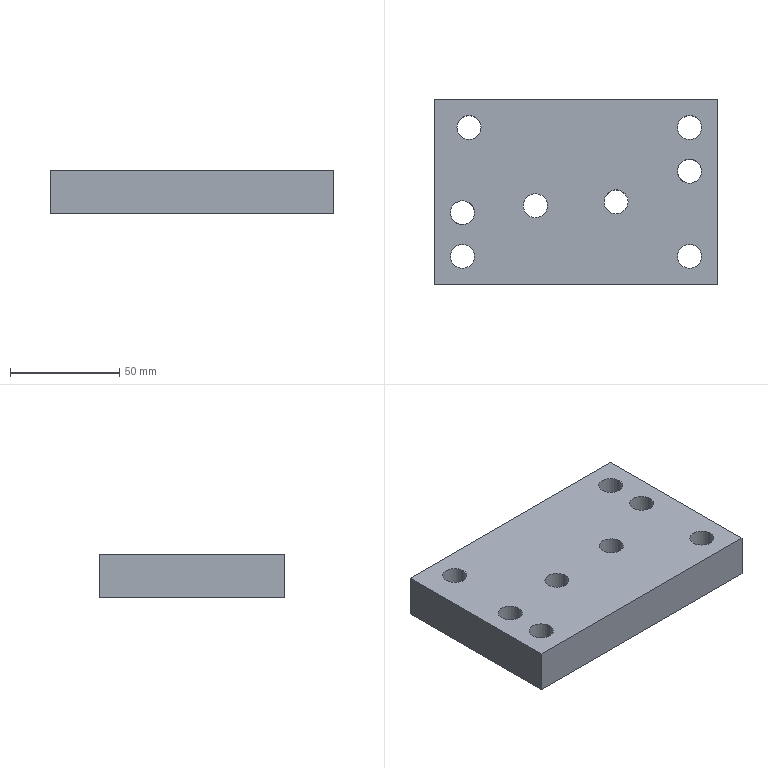Part | STEP file | 116_id2778_x_t | 1 solid | 14 faces | box 130 x 85 x 20 mm | volume 205795 mm3 | cylinder 8 | plane 6 | commonest cylinder face diameters 11 x8
STEP:
#1=CARTESIAN_POINT('',(0.,0.,0.));
#2=DIRECTION('',(0.,0.,1.));
#3=DIRECTION('',(1.,0.,0.));
#4=AXIS2_PLACEMENT_3D('',#1,#2,#3);
#5=CARTESIAN_POINT('',(1175.9,125.226,85.));
#6=VERTEX_POINT('',#5);
#7=CARTESIAN_POINT('',(1164.9,125.226,85.));
#8=VERTEX_POINT('',#7);
#9=CARTESIAN_POINT('',(1170.4,125.226,85.));
#10=DIRECTION('',(0.,0.,-1.));
#11=DIRECTION('',(-1.,0.,0.));
#12=AXIS2_PLACEMENT_3D('',#9,#10,#11);
#13=CIRCLE('',#12,5.5);
#14=CARTESIAN_POINT('',(1170.4,125.226,137.));
#15=DIRECTION('',(0.,0.,-1.));
#16=DIRECTION('',(1.,0.,0.));
#17=AXIS2_PLACEMENT_3D('',#14,#15,#16);
#18=CYLINDRICAL_SURFACE('',#17,5.5);
#19=CARTESIAN_POINT('',(-3.142,52.));
#20=DIRECTION('',(1.,0.));
#21=VECTOR('',#20,1.);
#22=LINE('',#19,#21);
#23=(GEOMETRIC_REPRESENTATION_CONTEXT(2)PARAMETRIC_REPRESENTATION_CONTEXT()REPRESENTATION_CONTEXT('',''));
#24=DEFINITIONAL_REPRESENTATION('',(#22),#23);
#25=PCURVE('',#18,#24);
#26=CARTESIAN_POINT('',(1128.,155.,85.));
#27=DIRECTION('',(0.,0.,-1.));
#28=DIRECTION('',(1.,0.,0.));
#29=AXIS2_PLACEMENT_3D('',#26,#27,#28);
#30=PLANE('',#29);
#31=CARTESIAN_POINT('',(42.4,29.774));
#32=DIRECTION('',(-1.,0.));
#33=AXIS2_PLACEMENT_2D('',#31,#32);
#34=CIRCLE('',#33,5.5);
#35=(GEOMETRIC_REPRESENTATION_CONTEXT(2)PARAMETRIC_REPRESENTATION_CONTEXT()REPRESENTATION_CONTEXT('',''));
#36=DEFINITIONAL_REPRESENTATION('',(#34),#35);
#37=PCURVE('',#30,#36);
#38=SURFACE_CURVE('',#13,(#25,#37),.PCURVE_S1.);
#39=EDGE_CURVE('',#6,#8,#38,.T.);
#40=ORIENTED_EDGE('',*,*,#39,.F.);
#41=CARTESIAN_POINT('',(1175.9,125.226,105.));
#42=VERTEX_POINT('',#41);
#43=CARTESIAN_POINT('',(1175.9,125.226,105.));
#44=CARTESIAN_POINT('',(1175.9,125.226,85.));
#45=B_SPLINE_CURVE_WITH_KNOTS('',1,(#43,#44),.UNSPECIFIED.,.F.,.F.,(2,2),(32.,52.),.PIECEWISE_BEZIER_KNOTS.);
#46=CARTESIAN_POINT('',(0.,0.));
#47=DIRECTION('',(0.,1.));
#48=VECTOR('',#47,1.);
#49=LINE('',#46,#48);
#50=(GEOMETRIC_REPRESENTATION_CONTEXT(2)PARAMETRIC_REPRESENTATION_CONTEXT()REPRESENTATION_CONTEXT('',''));
#51=DEFINITIONAL_REPRESENTATION('',(#49),#50);
#52=PCURVE('',#18,#51);
#53=CARTESIAN_POINT('',(6.283,0.));
#54=DIRECTION('',(0.,1.));
#55=VECTOR('',#54,1.);
#56=LINE('',#53,#55);
#57=(GEOMETRIC_REPRESENTATION_CONTEXT(2)PARAMETRIC_REPRESENTATION_CONTEXT()REPRESENTATION_CONTEXT('',''));
#58=DEFINITIONAL_REPRESENTATION('',(#56),#57);
#59=PCURVE('',#18,#58);
#60=SEAM_CURVE('',#45,(#52,#59),.PCURVE_S1.);
#61=EDGE_CURVE('',#42,#6,#60,.T.);
#62=ORIENTED_EDGE('',*,*,#61,.F.);
#63=CARTESIAN_POINT('',(1170.4,125.226,105.));
#64=DIRECTION('',(0.,0.,1.));
#65=DIRECTION('',(1.,0.,0.));
#66=AXIS2_PLACEMENT_3D('',#63,#64,#65);
#67=CIRCLE('',#66,5.5);
#68=CARTESIAN_POINT('',(6.283,32.));
#69=DIRECTION('',(-1.,0.));
#70=VECTOR('',#69,1.);
#71=LINE('',#68,#70);
#72=(GEOMETRIC_REPRESENTATION_CONTEXT(2)PARAMETRIC_REPRESENTATION_CONTEXT()REPRESENTATION_CONTEXT('',''));
#73=DEFINITIONAL_REPRESENTATION('',(#71),#72);
#74=PCURVE('',#18,#73);
#75=CARTESIAN_POINT('',(1128.,155.,105.));
#76=DIRECTION('',(0.,0.,1.));
#77=DIRECTION('',(-1.,0.,0.));
#78=AXIS2_PLACEMENT_3D('',#75,#76,#77);
#79=PLANE('',#78);
#80=CARTESIAN_POINT('',(-42.4,29.774));
#81=DIRECTION('',(-1.,0.));
#82=AXIS2_PLACEMENT_2D('',#80,#81);
#83=CIRCLE('',#82,5.5);
#84=(GEOMETRIC_REPRESENTATION_CONTEXT(2)PARAMETRIC_REPRESENTATION_CONTEXT()REPRESENTATION_CONTEXT('',''));
#85=DEFINITIONAL_REPRESENTATION('',(#83),#84);
#86=PCURVE('',#79,#85);
#87=SURFACE_CURVE('',#67,(#74,#86),.PCURVE_S1.);
#88=EDGE_CURVE('',#42,#42,#87,.T.);
#89=ORIENTED_EDGE('',*,*,#88,.F.);
#90=ORIENTED_EDGE('',*,*,#61,.T.);
#91=CARTESIAN_POINT('',(1170.4,125.226,85.));
#92=DIRECTION('',(0.,0.,-1.));
#93=DIRECTION('',(-1.,0.,0.));
#94=AXIS2_PLACEMENT_3D('',#91,#92,#93);
#95=CIRCLE('',#94,5.5);
#96=CARTESIAN_POINT('',(3.142,52.));
#97=DIRECTION('',(1.,0.));
#98=VECTOR('',#97,1.);
#99=LINE('',#96,#98);
#100=(GEOMETRIC_REPRESENTATION_CONTEXT(2)PARAMETRIC_REPRESENTATION_CONTEXT()REPRESENTATION_CONTEXT('',''));
#101=DEFINITIONAL_REPRESENTATION('',(#99),#100);
#102=PCURVE('',#18,#101);
#103=CARTESIAN_POINT('',(42.4,29.774));
#104=DIRECTION('',(-1.,0.));
#105=AXIS2_PLACEMENT_2D('',#103,#104);
#106=CIRCLE('',#105,5.5);
#107=(GEOMETRIC_REPRESENTATION_CONTEXT(2)PARAMETRIC_REPRESENTATION_CONTEXT()REPRESENTATION_CONTEXT('',''));
#108=DEFINITIONAL_REPRESENTATION('',(#106),#107);
#109=PCURVE('',#30,#108);
#110=SURFACE_CURVE('',#95,(#102,#109),.PCURVE_S1.);
#111=EDGE_CURVE('',#8,#6,#110,.T.);
#112=ORIENTED_EDGE('',*,*,#111,.F.);
#113=EDGE_LOOP('',(#40,#62,#89,#90,#112));
#114=FACE_BOUND('',#113,.F.);
#115=ADVANCED_FACE('',(#114),#18,.F.);
#116=CARTESIAN_POINT('',(1212.857,126.948,105.));
#117=VERTEX_POINT('',#116);
#118=CARTESIAN_POINT('',(1207.357,126.948,105.));
#119=DIRECTION('',(0.,0.,1.));
#120=DIRECTION('',(1.,0.,0.));
#121=AXIS2_PLACEMENT_3D('',#118,#119,#120);
#122=CIRCLE('',#121,5.5);
#123=CARTESIAN_POINT('',(1207.357,126.948,-13.));
#124=DIRECTION('',(0.,0.,1.));
#125=DIRECTION('',(0.9999,0.0167,0.));
#126=AXIS2_PLACEMENT_3D('',#123,#124,#125);
#127=CYLINDRICAL_SURFACE('',#126,5.5);
#128=CARTESIAN_POINT('',(6.266,118.));
#129=DIRECTION('',(1.,0.));
#130=VECTOR('',#129,1.);
#131=LINE('',#128,#130);
#132=(GEOMETRIC_REPRESENTATION_CONTEXT(2)PARAMETRIC_REPRESENTATION_CONTEXT()REPRESENTATION_CONTEXT('',''));
#133=DEFINITIONAL_REPRESENTATION('',(#131),#132);
#134=PCURVE('',#127,#133);
#135=CARTESIAN_POINT('',(-79.357,28.052));
#136=DIRECTION('',(-1.,0.));
#137=AXIS2_PLACEMENT_2D('',#135,#136);
#138=CIRCLE('',#137,5.5);
#139=(GEOMETRIC_REPRESENTATION_CONTEXT(2)PARAMETRIC_REPRESENTATION_CONTEXT()REPRESENTATION_CONTEXT('',''));
#140=DEFINITIONAL_REPRESENTATION('',(#138),#139);
#141=PCURVE('',#79,#140);
#142=SURFACE_CURVE('',#122,(#134,#141),.PCURVE_S1.);
#143=EDGE_CURVE('',#117,#117,#142,.T.);
#144=ORIENTED_EDGE('',*,*,#143,.F.);
#145=CARTESIAN_POINT('',(1212.857,126.948,85.));
#146=VERTEX_POINT('',#145);
#147=CARTESIAN_POINT('',(1212.857,126.948,85.));
#148=CARTESIAN_POINT('',(1212.857,126.948,105.));
#149=B_SPLINE_CURVE_WITH_KNOTS('',1,(#147,#148),.UNSPECIFIED.,.F.,.F.,(2,2),(98.,118.),.PIECEWISE_BEZIER_KNOTS.);
#150=CARTESIAN_POINT('',(6.266,0.));
#151=DIRECTION('',(0.,1.));
#152=VECTOR('',#151,1.);
#153=LINE('',#150,#152);
#154=(GEOMETRIC_REPRESENTATION_CONTEXT(2)PARAMETRIC_REPRESENTATION_CONTEXT()REPRESENTATION_CONTEXT('',''));
#155=DEFINITIONAL_REPRESENTATION('',(#153),#154);
#156=PCURVE('',#127,#155);
#157=CARTESIAN_POINT('',(12.55,0.));
#158=DIRECTION('',(0.,1.));
#159=VECTOR('',#158,1.);
#160=LINE('',#157,#159);
#161=(GEOMETRIC_REPRESENTATION_CONTEXT(2)PARAMETRIC_REPRESENTATION_CONTEXT()REPRESENTATION_CONTEXT('',''));
#162=DEFINITIONAL_REPRESENTATION('',(#160),#161);
#163=PCURVE('',#127,#162);
#164=SEAM_CURVE('',#149,(#156,#163),.PCURVE_S1.);
#165=EDGE_CURVE('',#146,#117,#164,.T.);
#166=ORIENTED_EDGE('',*,*,#165,.F.);
#167=CARTESIAN_POINT('',(1201.857,126.948,85.));
#168=VERTEX_POINT('',#167);
#169=CARTESIAN_POINT('',(1207.357,126.948,85.));
#170=DIRECTION('',(0.,0.,-1.));
#171=DIRECTION('',(-1.,0.,0.));
#172=AXIS2_PLACEMENT_3D('',#169,#170,#171);
#173=CIRCLE('',#172,5.5);
#174=CARTESIAN_POINT('',(9.408,98.));
#175=DIRECTION('',(-1.,0.));
#176=VECTOR('',#175,1.);
#177=LINE('',#174,#176);
#178=(GEOMETRIC_REPRESENTATION_CONTEXT(2)PARAMETRIC_REPRESENTATION_CONTEXT()REPRESENTATION_CONTEXT('',''));
#179=DEFINITIONAL_REPRESENTATION('',(#177),#178);
#180=PCURVE('',#127,#179);
#181=CARTESIAN_POINT('',(79.357,28.052));
#182=DIRECTION('',(-1.,0.));
#183=AXIS2_PLACEMENT_2D('',#181,#182);
#184=CIRCLE('',#183,5.5);
#185=(GEOMETRIC_REPRESENTATION_CONTEXT(2)PARAMETRIC_REPRESENTATION_CONTEXT()REPRESENTATION_CONTEXT('',''));
#186=DEFINITIONAL_REPRESENTATION('',(#184),#185);
#187=PCURVE('',#30,#186);
#188=SURFACE_CURVE('',#173,(#180,#187),.PCURVE_S1.);
#189=EDGE_CURVE('',#168,#146,#188,.T.);
#190=ORIENTED_EDGE('',*,*,#189,.F.);
#191=CARTESIAN_POINT('',(1207.357,126.948,85.));
#192=DIRECTION('',(0.,0.,-1.));
#193=DIRECTION('',(-1.,0.,0.));
#194=AXIS2_PLACEMENT_3D('',#191,#192,#193);
#195=CIRCLE('',#194,5.5);
#196=CARTESIAN_POINT('',(15.691,98.));
#197=DIRECTION('',(-1.,0.));
#198=VECTOR('',#197,1.);
#199=LINE('',#196,#198);
#200=(GEOMETRIC_REPRESENTATION_CONTEXT(2)PARAMETRIC_REPRESENTATION_CONTEXT()REPRESENTATION_CONTEXT('',''));
#201=DEFINITIONAL_REPRESENTATION('',(#199),#200);
#202=PCURVE('',#127,#201);
#203=CARTESIAN_POINT('',(79.357,28.052));
#204=DIRECTION('',(-1.,0.));
#205=AXIS2_PLACEMENT_2D('',#203,#204);
#206=CIRCLE('',#205,5.5);
#207=(GEOMETRIC_REPRESENTATION_CONTEXT(2)PARAMETRIC_REPRESENTATION_CONTEXT()REPRESENTATION_CONTEXT('',''));
#208=DEFINITIONAL_REPRESENTATION('',(#206),#207);
#209=PCURVE('',#30,#208);
#210=SURFACE_CURVE('',#195,(#202,#209),.PCURVE_S1.);
#211=EDGE_CURVE('',#146,#168,#210,.T.);
#212=ORIENTED_EDGE('',*,*,#211,.F.);
#213=ORIENTED_EDGE('',*,*,#165,.T.);
#214=EDGE_LOOP('',(#144,#166,#190,#212,#213));
#215=FACE_BOUND('',#214,.F.);
#216=ADVANCED_FACE('',(#215),#127,.F.);
#217=CARTESIAN_POINT('',(1124.,174.,105.));
#218=VERTEX_POINT('',#217);
#219=CARTESIAN_POINT('',(1254.,174.,105.));
#220=VERTEX_POINT('',#219);
#221=CARTESIAN_POINT('',(1128.,174.,105.));
#222=DIRECTION('',(1.,0.,0.));
#223=VECTOR('',#222,1.);
#224=LINE('',#221,#223);
#225=CARTESIAN_POINT('',(1128.,174.,90.));
#226=DIRECTION('',(0.,1.,0.));
#227=DIRECTION('',(0.,0.,-1.));
#228=AXIS2_PLACEMENT_3D('',#225,#226,#227);
#229=PLANE('',#228);
#230=CARTESIAN_POINT('',(-15.,0.));
#231=DIRECTION('',(0.,-1.));
#232=VECTOR('',#231,1.);
#233=LINE('',#230,#232);
#234=(GEOMETRIC_REPRESENTATION_CONTEXT(2)PARAMETRIC_REPRESENTATION_CONTEXT()REPRESENTATION_CONTEXT('',''));
#235=DEFINITIONAL_REPRESENTATION('',(#233),#234);
#236=PCURVE('',#229,#235);
#237=CARTESIAN_POINT('',(0.,-19.));
#238=DIRECTION('',(-1.,0.));
#239=VECTOR('',#238,1.);
#240=LINE('',#237,#239);
#241=(GEOMETRIC_REPRESENTATION_CONTEXT(2)PARAMETRIC_REPRESENTATION_CONTEXT()REPRESENTATION_CONTEXT('',''));
#242=DEFINITIONAL_REPRESENTATION('',(#240),#241);
#243=PCURVE('',#79,#242);
#244=SURFACE_CURVE('',#224,(#236,#243),.PCURVE_S1.);
#245=EDGE_CURVE('',#218,#220,#244,.T.);
#246=ORIENTED_EDGE('',*,*,#245,.T.);
#247=CARTESIAN_POINT('',(1254.,174.,85.));
#248=VERTEX_POINT('',#247);
#249=CARTESIAN_POINT('',(1254.,174.,90.));
#250=DIRECTION('',(0.,0.,1.));
#251=VECTOR('',#250,1.);
#252=LINE('',#249,#251);
#253=CARTESIAN_POINT('',(0.,-126.));
#254=DIRECTION('',(-1.,0.));
#255=VECTOR('',#254,1.);
#256=LINE('',#253,#255);
#257=(GEOMETRIC_REPRESENTATION_CONTEXT(2)PARAMETRIC_REPRESENTATION_CONTEXT()REPRESENTATION_CONTEXT('',''));
#258=DEFINITIONAL_REPRESENTATION('',(#256),#257);
#259=PCURVE('',#229,#258);
#260=CARTESIAN_POINT('',(1254.,155.,90.));
#261=DIRECTION('',(1.,0.,0.));
#262=DIRECTION('',(0.,0.,1.));
#263=AXIS2_PLACEMENT_3D('',#260,#261,#262);
#264=PLANE('',#263);
#265=CARTESIAN_POINT('',(0.,-19.));
#266=DIRECTION('',(1.,0.));
#267=VECTOR('',#266,1.);
#268=LINE('',#265,#267);
#269=(GEOMETRIC_REPRESENTATION_CONTEXT(2)PARAMETRIC_REPRESENTATION_CONTEXT()REPRESENTATION_CONTEXT('',''));
#270=DEFINITIONAL_REPRESENTATION('',(#268),#269);
#271=PCURVE('',#264,#270);
#272=SURFACE_CURVE('',#252,(#259,#271),.PCURVE_S1.);
#273=EDGE_CURVE('',#248,#220,#272,.T.);
#274=ORIENTED_EDGE('',*,*,#273,.F.);
#275=CARTESIAN_POINT('',(1124.,174.,85.));
#276=VERTEX_POINT('',#275);
#277=CARTESIAN_POINT('',(1128.,174.,85.));
#278=DIRECTION('',(-1.,0.,0.));
#279=VECTOR('',#278,1.);
#280=LINE('',#277,#279);
#281=CARTESIAN_POINT('',(5.,0.));
#282=DIRECTION('',(0.,1.));
#283=VECTOR('',#282,1.);
#284=LINE('',#281,#283);
#285=(GEOMETRIC_REPRESENTATION_CONTEXT(2)PARAMETRIC_REPRESENTATION_CONTEXT()REPRESENTATION_CONTEXT('',''));
#286=DEFINITIONAL_REPRESENTATION('',(#284),#285);
#287=PCURVE('',#229,#286);
#288=CARTESIAN_POINT('',(0.,-19.));
#289=DIRECTION('',(-1.,0.));
#290=VECTOR('',#289,1.);
#291=LINE('',#288,#290);
#292=(GEOMETRIC_REPRESENTATION_CONTEXT(2)PARAMETRIC_REPRESENTATION_CONTEXT()REPRESENTATION_CONTEXT('',''));
#293=DEFINITIONAL_REPRESENTATION('',(#291),#292);
#294=PCURVE('',#30,#293);
#295=SURFACE_CURVE('',#280,(#287,#294),.PCURVE_S1.);
#296=EDGE_CURVE('',#248,#276,#295,.T.);
#297=ORIENTED_EDGE('',*,*,#296,.T.);
#298=CARTESIAN_POINT('',(1124.,174.,90.));
#299=DIRECTION('',(0.,0.,-1.));
#300=VECTOR('',#299,1.);
#301=LINE('',#298,#300);
#302=CARTESIAN_POINT('',(0.,4.));
#303=DIRECTION('',(1.,0.));
#304=VECTOR('',#303,1.);
#305=LINE('',#302,#304);
#306=(GEOMETRIC_REPRESENTATION_CONTEXT(2)PARAMETRIC_REPRESENTATION_CONTEXT()REPRESENTATION_CONTEXT('',''));
#307=DEFINITIONAL_REPRESENTATION('',(#305),#306);
#308=PCURVE('',#229,#307);
#309=CARTESIAN_POINT('',(1124.,108.,90.));
#310=DIRECTION('',(-1.,0.,0.));
#311=DIRECTION('',(0.,0.,1.));
#312=AXIS2_PLACEMENT_3D('',#309,#310,#311);
#313=PLANE('',#312);
#314=CARTESIAN_POINT('',(0.,66.));
#315=DIRECTION('',(-1.,0.));
#316=VECTOR('',#315,1.);
#317=LINE('',#314,#316);
#318=(GEOMETRIC_REPRESENTATION_CONTEXT(2)PARAMETRIC_REPRESENTATION_CONTEXT()REPRESENTATION_CONTEXT('',''));
#319=DEFINITIONAL_REPRESENTATION('',(#317),#318);
#320=PCURVE('',#313,#319);
#321=SURFACE_CURVE('',#301,(#308,#320),.PCURVE_S1.);
#322=EDGE_CURVE('',#218,#276,#321,.T.);
#323=ORIENTED_EDGE('',*,*,#322,.F.);
#324=EDGE_LOOP('',(#246,#274,#297,#323));
#325=FACE_BOUND('',#324,.T.);
#326=ADVANCED_FACE('',(#325),#229,.T.);
#327=CARTESIAN_POINT('',(1124.,89.,85.));
#328=VERTEX_POINT('',#327);
#329=CARTESIAN_POINT('',(1254.,89.,85.));
#330=VERTEX_POINT('',#329);
#331=CARTESIAN_POINT('',(1128.,89.,85.));
#332=DIRECTION('',(1.,0.,0.));
#333=VECTOR('',#332,1.);
#334=LINE('',#331,#333);
#335=CARTESIAN_POINT('',(1128.,89.,90.));
#336=DIRECTION('',(0.,-1.,0.));
#337=DIRECTION('',(0.,0.,1.));
#338=AXIS2_PLACEMENT_3D('',#335,#336,#337);
#339=PLANE('',#338);
#340=CARTESIAN_POINT('',(-5.,0.));
#341=DIRECTION('',(0.,-1.));
#342=VECTOR('',#341,1.);
#343=LINE('',#340,#342);
#344=(GEOMETRIC_REPRESENTATION_CONTEXT(2)PARAMETRIC_REPRESENTATION_CONTEXT()REPRESENTATION_CONTEXT('',''));
#345=DEFINITIONAL_REPRESENTATION('',(#343),#344);
#346=PCURVE('',#339,#345);
#347=CARTESIAN_POINT('',(0.,66.));
#348=DIRECTION('',(1.,0.));
#349=VECTOR('',#348,1.);
#350=LINE('',#347,#349);
#351=(GEOMETRIC_REPRESENTATION_CONTEXT(2)PARAMETRIC_REPRESENTATION_CONTEXT()REPRESENTATION_CONTEXT('',''));
#352=DEFINITIONAL_REPRESENTATION('',(#350),#351);
#353=PCURVE('',#30,#352);
#354=SURFACE_CURVE('',#334,(#346,#353),.PCURVE_S1.);
#355=EDGE_CURVE('',#328,#330,#354,.T.);
#356=ORIENTED_EDGE('',*,*,#355,.T.);
#357=CARTESIAN_POINT('',(1254.,89.,105.));
#358=VERTEX_POINT('',#357);
#359=CARTESIAN_POINT('',(1254.,89.,90.));
#360=DIRECTION('',(0.,0.,1.));
#361=VECTOR('',#360,1.);
#362=LINE('',#359,#361);
#363=CARTESIAN_POINT('',(0.,-126.));
#364=DIRECTION('',(1.,0.));
#365=VECTOR('',#364,1.);
#366=LINE('',#363,#365);
#367=(GEOMETRIC_REPRESENTATION_CONTEXT(2)PARAMETRIC_REPRESENTATION_CONTEXT()REPRESENTATION_CONTEXT('',''));
#368=DEFINITIONAL_REPRESENTATION('',(#366),#367);
#369=PCURVE('',#339,#368);
#370=CARTESIAN_POINT('',(0.,66.));
#371=DIRECTION('',(1.,0.));
#372=VECTOR('',#371,1.);
#373=LINE('',#370,#372);
#374=(GEOMETRIC_REPRESENTATION_CONTEXT(2)PARAMETRIC_REPRESENTATION_CONTEXT()REPRESENTATION_CONTEXT('',''));
#375=DEFINITIONAL_REPRESENTATION('',(#373),#374);
#376=PCURVE('',#264,#375);
#377=SURFACE_CURVE('',#362,(#369,#376),.PCURVE_S1.);
#378=EDGE_CURVE('',#330,#358,#377,.T.);
#379=ORIENTED_EDGE('',*,*,#378,.T.);
#380=CARTESIAN_POINT('',(1124.,89.,105.));
#381=VERTEX_POINT('',#380);
#382=CARTESIAN_POINT('',(1128.,89.,105.));
#383=DIRECTION('',(-1.,0.,0.));
#384=VECTOR('',#383,1.);
#385=LINE('',#382,#384);
#386=CARTESIAN_POINT('',(15.,0.));
#387=DIRECTION('',(0.,1.));
#388=VECTOR('',#387,1.);
#389=LINE('',#386,#388);
#390=(GEOMETRIC_REPRESENTATION_CONTEXT(2)PARAMETRIC_REPRESENTATION_CONTEXT()REPRESENTATION_CONTEXT('',''));
#391=DEFINITIONAL_REPRESENTATION('',(#389),#390);
#392=PCURVE('',#339,#391);
#393=CARTESIAN_POINT('',(0.,66.));
#394=DIRECTION('',(1.,0.));
#395=VECTOR('',#394,1.);
#396=LINE('',#393,#395);
#397=(GEOMETRIC_REPRESENTATION_CONTEXT(2)PARAMETRIC_REPRESENTATION_CONTEXT()REPRESENTATION_CONTEXT('',''));
#398=DEFINITIONAL_REPRESENTATION('',(#396),#397);
#399=PCURVE('',#79,#398);
#400=SURFACE_CURVE('',#385,(#392,#399),.PCURVE_S1.);
#401=EDGE_CURVE('',#358,#381,#400,.T.);
#402=ORIENTED_EDGE('',*,*,#401,.T.);
#403=CARTESIAN_POINT('',(1124.,89.,90.));
#404=DIRECTION('',(0.,0.,-1.));
#405=VECTOR('',#404,1.);
#406=LINE('',#403,#405);
#407=CARTESIAN_POINT('',(0.,4.));
#408=DIRECTION('',(-1.,0.));
#409=VECTOR('',#408,1.);
#410=LINE('',#407,#409);
#411=(GEOMETRIC_REPRESENTATION_CONTEXT(2)PARAMETRIC_REPRESENTATION_CONTEXT()REPRESENTATION_CONTEXT('',''));
#412=DEFINITIONAL_REPRESENTATION('',(#410),#411);
#413=PCURVE('',#339,#412);
#414=CARTESIAN_POINT('',(0.,-19.));
#415=DIRECTION('',(-1.,0.));
#416=VECTOR('',#415,1.);
#417=LINE('',#414,#416);
#418=(GEOMETRIC_REPRESENTATION_CONTEXT(2)PARAMETRIC_REPRESENTATION_CONTEXT()REPRESENTATION_CONTEXT('',''));
#419=DEFINITIONAL_REPRESENTATION('',(#417),#418);
#420=PCURVE('',#313,#419);
#421=SURFACE_CURVE('',#406,(#413,#420),.PCURVE_S1.);
#422=EDGE_CURVE('',#381,#328,#421,.T.);
#423=ORIENTED_EDGE('',*,*,#422,.T.);
#424=EDGE_LOOP('',(#356,#379,#402,#423));
#425=FACE_BOUND('',#424,.T.);
#426=ADVANCED_FACE('',(#425),#339,.T.);
#427=ORIENTED_EDGE('',*,*,#143,.F.);
#428=EDGE_LOOP('',(#427));
#429=FACE_BOUND('',#428,.T.);
#430=ORIENTED_EDGE('',*,*,#88,.F.);
#431=EDGE_LOOP('',(#430));
#432=FACE_BOUND('',#431,.T.);
#433=ORIENTED_EDGE('',*,*,#401,.F.);
#434=CARTESIAN_POINT('',(1254.,155.,105.));
#435=DIRECTION('',(0.,-1.,0.));
#436=VECTOR('',#435,1.);
#437=LINE('',#434,#436);
#438=CARTESIAN_POINT('',(-126.,0.));
#439=DIRECTION('',(0.,1.));
#440=VECTOR('',#439,1.);
#441=LINE('',#438,#440);
#442=(GEOMETRIC_REPRESENTATION_CONTEXT(2)PARAMETRIC_REPRESENTATION_CONTEXT()REPRESENTATION_CONTEXT('',''));
#443=DEFINITIONAL_REPRESENTATION('',(#441),#442);
#444=PCURVE('',#79,#443);
#445=CARTESIAN_POINT('',(15.,0.));
#446=DIRECTION('',(0.,1.));
#447=VECTOR('',#446,1.);
#448=LINE('',#445,#447);
#449=(GEOMETRIC_REPRESENTATION_CONTEXT(2)PARAMETRIC_REPRESENTATION_CONTEXT()REPRESENTATION_CONTEXT('',''));
#450=DEFINITIONAL_REPRESENTATION('',(#448),#449);
#451=PCURVE('',#264,#450);
#452=SURFACE_CURVE('',#437,(#444,#451),.PCURVE_S1.);
#453=EDGE_CURVE('',#220,#358,#452,.T.);
#454=ORIENTED_EDGE('',*,*,#453,.F.);
#455=ORIENTED_EDGE('',*,*,#245,.F.);
#456=CARTESIAN_POINT('',(1124.,155.,105.));
#457=DIRECTION('',(0.,-1.,0.));
#458=VECTOR('',#457,1.);
#459=LINE('',#456,#458);
#460=CARTESIAN_POINT('',(4.,0.));
#461=DIRECTION('',(0.,1.));
#462=VECTOR('',#461,1.);
#463=LINE('',#460,#462);
#464=(GEOMETRIC_REPRESENTATION_CONTEXT(2)PARAMETRIC_REPRESENTATION_CONTEXT()REPRESENTATION_CONTEXT('',''));
#465=DEFINITIONAL_REPRESENTATION('',(#463),#464);
#466=PCURVE('',#79,#465);
#467=CARTESIAN_POINT('',(15.,47.));
#468=DIRECTION('',(0.,-1.));
#469=VECTOR('',#468,1.);
#470=LINE('',#467,#469);
#471=(GEOMETRIC_REPRESENTATION_CONTEXT(2)PARAMETRIC_REPRESENTATION_CONTEXT()REPRESENTATION_CONTEXT('',''));
#472=DEFINITIONAL_REPRESENTATION('',(#470),#471);
#473=PCURVE('',#313,#472);
#474=SURFACE_CURVE('',#459,(#466,#473),.PCURVE_S1.);
#475=EDGE_CURVE('',#218,#381,#474,.T.);
#476=ORIENTED_EDGE('',*,*,#475,.T.);
#477=EDGE_LOOP('',(#433,#454,#455,#476));
#478=FACE_BOUND('',#477,.T.);
#479=CARTESIAN_POINT('',(1134.5,161.,105.));
#480=VERTEX_POINT('',#479);
#481=CARTESIAN_POINT('',(1140.,161.,105.));
#482=DIRECTION('',(0.,0.,1.));
#483=DIRECTION('',(1.,0.,0.));
#484=AXIS2_PLACEMENT_3D('',#481,#482,#483);
#485=CIRCLE('',#484,5.5);
#486=CARTESIAN_POINT('',(-12.,-6.));
#487=DIRECTION('',(-1.,0.));
#488=AXIS2_PLACEMENT_2D('',#486,#487);
#489=CIRCLE('',#488,5.5);
#490=(GEOMETRIC_REPRESENTATION_CONTEXT(2)PARAMETRIC_REPRESENTATION_CONTEXT()REPRESENTATION_CONTEXT('',''));
#491=DEFINITIONAL_REPRESENTATION('',(#489),#490);
#492=PCURVE('',#79,#491);
#493=CARTESIAN_POINT('',(1140.,161.,90.));
#494=DIRECTION('',(0.,0.,1.));
#495=DIRECTION('',(1.,0.,0.));
#496=AXIS2_PLACEMENT_3D('',#493,#494,#495);
#497=CYLINDRICAL_SURFACE('',#496,5.5);
#498=CARTESIAN_POINT('',(0.,15.));
#499=DIRECTION('',(1.,0.));
#500=VECTOR('',#499,1.);
#501=LINE('',#498,#500);
#502=(GEOMETRIC_REPRESENTATION_CONTEXT(2)PARAMETRIC_REPRESENTATION_CONTEXT()REPRESENTATION_CONTEXT('',''));
#503=DEFINITIONAL_REPRESENTATION('',(#501),#502);
#504=PCURVE('',#497,#503);
#505=SURFACE_CURVE('',#485,(#492,#504),.PCURVE_S1.);
#506=EDGE_CURVE('',#480,#480,#505,.T.);
#507=ORIENTED_EDGE('',*,*,#506,.F.);
#508=EDGE_LOOP('',(#507));
#509=FACE_BOUND('',#508,.T.);
#510=CARTESIAN_POINT('',(1131.5,102.,105.));
#511=VERTEX_POINT('',#510);
#512=CARTESIAN_POINT('',(1137.,102.,105.));
#513=DIRECTION('',(0.,0.,1.));
#514=DIRECTION('',(1.,0.,0.));
#515=AXIS2_PLACEMENT_3D('',#512,#513,#514);
#516=CIRCLE('',#515,5.5);
#517=CARTESIAN_POINT('',(-9.,53.));
#518=DIRECTION('',(-1.,0.));
#519=AXIS2_PLACEMENT_2D('',#517,#518);
#520=CIRCLE('',#519,5.5);
#521=(GEOMETRIC_REPRESENTATION_CONTEXT(2)PARAMETRIC_REPRESENTATION_CONTEXT()REPRESENTATION_CONTEXT('',''));
#522=DEFINITIONAL_REPRESENTATION('',(#520),#521);
#523=PCURVE('',#79,#522);
#524=CARTESIAN_POINT('',(1137.,102.,90.));
#525=DIRECTION('',(0.,0.,1.));
#526=DIRECTION('',(1.,0.,0.));
#527=AXIS2_PLACEMENT_3D('',#524,#525,#526);
#528=CYLINDRICAL_SURFACE('',#527,5.5);
#529=CARTESIAN_POINT('',(0.,15.));
#530=DIRECTION('',(1.,0.));
#531=VECTOR('',#530,1.);
#532=LINE('',#529,#531);
#533=(GEOMETRIC_REPRESENTATION_CONTEXT(2)PARAMETRIC_REPRESENTATION_CONTEXT()REPRESENTATION_CONTEXT('',''));
#534=DEFINITIONAL_REPRESENTATION('',(#532),#533);
#535=PCURVE('',#528,#534);
#536=SURFACE_CURVE('',#516,(#523,#535),.PCURVE_S1.);
#537=EDGE_CURVE('',#511,#511,#536,.T.);
#538=ORIENTED_EDGE('',*,*,#537,.F.);
#539=EDGE_LOOP('',(#538));
#540=FACE_BOUND('',#539,.T.);
#541=CARTESIAN_POINT('',(1131.5,122.,105.));
#542=VERTEX_POINT('',#541);
#543=CARTESIAN_POINT('',(1137.,122.,105.));
#544=DIRECTION('',(0.,0.,1.));
#545=DIRECTION('',(1.,0.,0.));
#546=AXIS2_PLACEMENT_3D('',#543,#544,#545);
#547=CIRCLE('',#546,5.5);
#548=CARTESIAN_POINT('',(-9.,33.));
#549=DIRECTION('',(-1.,0.));
#550=AXIS2_PLACEMENT_2D('',#548,#549);
#551=CIRCLE('',#550,5.5);
#552=(GEOMETRIC_REPRESENTATION_CONTEXT(2)PARAMETRIC_REPRESENTATION_CONTEXT()REPRESENTATION_CONTEXT('',''));
#553=DEFINITIONAL_REPRESENTATION('',(#551),#552);
#554=PCURVE('',#79,#553);
#555=CARTESIAN_POINT('',(1137.,122.,90.));
#556=DIRECTION('',(0.,0.,1.));
#557=DIRECTION('',(0.,1.,0.));
#558=AXIS2_PLACEMENT_3D('',#555,#556,#557);
#559=CYLINDRICAL_SURFACE('',#558,5.5);
#560=CARTESIAN_POINT('',(-1.571,15.));
#561=DIRECTION('',(1.,0.));
#562=VECTOR('',#561,1.);
#563=LINE('',#560,#562);
#564=(GEOMETRIC_REPRESENTATION_CONTEXT(2)PARAMETRIC_REPRESENTATION_CONTEXT()REPRESENTATION_CONTEXT('',''));
#565=DEFINITIONAL_REPRESENTATION('',(#563),#564);
#566=PCURVE('',#559,#565);
#567=SURFACE_CURVE('',#547,(#554,#566),.PCURVE_S1.);
#568=EDGE_CURVE('',#542,#542,#567,.T.);
#569=ORIENTED_EDGE('',*,*,#568,.F.);
#570=EDGE_LOOP('',(#569));
#571=FACE_BOUND('',#570,.T.);
#572=CARTESIAN_POINT('',(1246.5,102.,105.));
#573=VERTEX_POINT('',#572);
#574=CARTESIAN_POINT('',(1241.,102.,105.));
#575=DIRECTION('',(0.,0.,-1.));
#576=DIRECTION('',(1.,0.,0.));
#577=AXIS2_PLACEMENT_3D('',#574,#575,#576);
#578=CIRCLE('',#577,5.5);
#579=CARTESIAN_POINT('',(-118.5,53.));
#580=CARTESIAN_POINT('',(-118.5,62.526));
#581=CARTESIAN_POINT('',(-110.25,57.763));
#582=CARTESIAN_POINT('',(-102.,53.));
#583=CARTESIAN_POINT('',(-110.25,48.237));
#584=CARTESIAN_POINT('',(-118.5,43.474));
#585=CARTESIAN_POINT('',(-118.5,53.));
#586=(BOUNDED_CURVE()B_SPLINE_CURVE(2,(#579,#580,#581,#582,#583,#584,#585),.UNSPECIFIED.,.T.,.F.)B_SPLINE_CURVE_WITH_KNOTS((1,2,2,2,2,1),(-2.094,0.,2.094,4.189,6.283,8.378),.UNSPECIFIED.)CURVE()GEOMETRIC_REPRESENTATION_ITEM()RATIONAL_B_SPLINE_CURVE((1.,0.5,1.,0.5,1.,0.5,1.))REPRESENTATION_ITEM(''));
#587=(GEOMETRIC_REPRESENTATION_CONTEXT(2)PARAMETRIC_REPRESENTATION_CONTEXT()REPRESENTATION_CONTEXT('',''));
#588=DEFINITIONAL_REPRESENTATION('',(#586),#587);
#589=PCURVE('',#79,#588);
#590=CARTESIAN_POINT('',(1241.,102.,90.));
#591=DIRECTION('',(0.,0.,1.));
#592=DIRECTION('',(-1.,0.,0.));
#593=AXIS2_PLACEMENT_3D('',#590,#591,#592);
#594=CYLINDRICAL_SURFACE('',#593,5.5);
#595=CARTESIAN_POINT('',(9.425,15.));
#596=DIRECTION('',(-1.,0.));
#597=VECTOR('',#596,1.);
#598=LINE('',#595,#597);
#599=(GEOMETRIC_REPRESENTATION_CONTEXT(2)PARAMETRIC_REPRESENTATION_CONTEXT()REPRESENTATION_CONTEXT('',''));
#600=DEFINITIONAL_REPRESENTATION('',(#598),#599);
#601=PCURVE('',#594,#600);
#602=SURFACE_CURVE('',#578,(#589,#601),.PCURVE_S1.);
#603=EDGE_CURVE('',#573,#573,#602,.T.);
#604=ORIENTED_EDGE('',*,*,#603,.T.);
#605=EDGE_LOOP('',(#604));
#606=FACE_BOUND('',#605,.T.);
#607=CARTESIAN_POINT('',(1246.5,161.,105.));
#608=VERTEX_POINT('',#607);
#609=CARTESIAN_POINT('',(1241.,161.,105.));
#610=DIRECTION('',(0.,0.,-1.));
#611=DIRECTION('',(1.,0.,0.));
#612=AXIS2_PLACEMENT_3D('',#609,#610,#611);
#613=CIRCLE('',#612,5.5);
#614=CARTESIAN_POINT('',(-118.5,-6.));
#615=CARTESIAN_POINT('',(-118.5,3.526));
#616=CARTESIAN_POINT('',(-110.25,-1.237));
#617=CARTESIAN_POINT('',(-102.,-6.));
#618=CARTESIAN_POINT('',(-110.25,-10.763));
#619=CARTESIAN_POINT('',(-118.5,-15.526));
#620=CARTESIAN_POINT('',(-118.5,-6.));
#621=(BOUNDED_CURVE()B_SPLINE_CURVE(2,(#614,#615,#616,#617,#618,#619,#620),.UNSPECIFIED.,.T.,.F.)B_SPLINE_CURVE_WITH_KNOTS((1,2,2,2,2,1),(-2.094,0.,2.094,4.189,6.283,8.378),.UNSPECIFIED.)CURVE()GEOMETRIC_REPRESENTATION_ITEM()RATIONAL_B_SPLINE_CURVE((1.,0.5,1.,0.5,1.,0.5,1.))REPRESENTATION_ITEM(''));
#622=(GEOMETRIC_REPRESENTATION_CONTEXT(2)PARAMETRIC_REPRESENTATION_CONTEXT()REPRESENTATION_CONTEXT('',''));
#623=DEFINITIONAL_REPRESENTATION('',(#621),#622);
#624=PCURVE('',#79,#623);
#625=CARTESIAN_POINT('',(1241.,161.,90.));
#626=DIRECTION('',(0.,0.,1.));
#627=DIRECTION('',(-1.,0.,0.));
#628=AXIS2_PLACEMENT_3D('',#625,#626,#627);
#629=CYLINDRICAL_SURFACE('',#628,5.5);
#630=CARTESIAN_POINT('',(9.425,15.));
#631=DIRECTION('',(-1.,0.));
#632=VECTOR('',#631,1.);
#633=LINE('',#630,#632);
#634=(GEOMETRIC_REPRESENTATION_CONTEXT(2)PARAMETRIC_REPRESENTATION_CONTEXT()REPRESENTATION_CONTEXT('',''));
#635=DEFINITIONAL_REPRESENTATION('',(#633),#634);
#636=PCURVE('',#629,#635);
#637=SURFACE_CURVE('',#613,(#624,#636),.PCURVE_S1.);
#638=EDGE_CURVE('',#608,#608,#637,.T.);
#639=ORIENTED_EDGE('',*,*,#638,.T.);
#640=EDGE_LOOP('',(#639));
#641=FACE_BOUND('',#640,.T.);
#642=CARTESIAN_POINT('',(1246.5,141.,105.));
#643=VERTEX_POINT('',#642);
#644=CARTESIAN_POINT('',(1241.,141.,105.));
#645=DIRECTION('',(0.,0.,-1.));
#646=DIRECTION('',(1.,0.,0.));
#647=AXIS2_PLACEMENT_3D('',#644,#645,#646);
#648=CIRCLE('',#647,5.5);
#649=CARTESIAN_POINT('',(-118.5,14.));
#650=CARTESIAN_POINT('',(-118.5,23.526));
#651=CARTESIAN_POINT('',(-110.25,18.763));
#652=CARTESIAN_POINT('',(-102.,14.));
#653=CARTESIAN_POINT('',(-110.25,9.237));
#654=CARTESIAN_POINT('',(-118.5,4.474));
#655=CARTESIAN_POINT('',(-118.5,14.));
#656=(BOUNDED_CURVE()B_SPLINE_CURVE(2,(#649,#650,#651,#652,#653,#654,#655),.UNSPECIFIED.,.T.,.F.)B_SPLINE_CURVE_WITH_KNOTS((1,2,2,2,2,1),(-2.094,0.,2.094,4.189,6.283,8.378),.UNSPECIFIED.)CURVE()GEOMETRIC_REPRESENTATION_ITEM()RATIONAL_B_SPLINE_CURVE((1.,0.5,1.,0.5,1.,0.5,1.))REPRESENTATION_ITEM(''));
#657=(GEOMETRIC_REPRESENTATION_CONTEXT(2)PARAMETRIC_REPRESENTATION_CONTEXT()REPRESENTATION_CONTEXT('',''));
#658=DEFINITIONAL_REPRESENTATION('',(#656),#657);
#659=PCURVE('',#79,#658);
#660=CARTESIAN_POINT('',(1241.,141.,90.));
#661=DIRECTION('',(0.,0.,1.));
#662=DIRECTION('',(0.,-1.,0.));
#663=AXIS2_PLACEMENT_3D('',#660,#661,#662);
#664=CYLINDRICAL_SURFACE('',#663,5.5);
#665=CARTESIAN_POINT('',(7.854,15.));
#666=DIRECTION('',(-1.,0.));
#667=VECTOR('',#666,1.);
#668=LINE('',#665,#667);
#669=(GEOMETRIC_REPRESENTATION_CONTEXT(2)PARAMETRIC_REPRESENTATION_CONTEXT()REPRESENTATION_CONTEXT('',''));
#670=DEFINITIONAL_REPRESENTATION('',(#668),#669);
#671=PCURVE('',#664,#670);
#672=SURFACE_CURVE('',#648,(#659,#671),.PCURVE_S1.);
#673=EDGE_CURVE('',#643,#643,#672,.T.);
#674=ORIENTED_EDGE('',*,*,#673,.T.);
#675=EDGE_LOOP('',(#674));
#676=FACE_BOUND('',#675,.T.);
#677=ADVANCED_FACE('',(#429,#432,#478,#509,#540,#571,#606,#641,#676),#79,.T.);
#678=ORIENTED_EDGE('',*,*,#189,.F.);
#679=ORIENTED_EDGE('',*,*,#211,.F.);
#680=EDGE_LOOP('',(#678,#679));
#681=FACE_BOUND('',#680,.T.);
#682=ORIENTED_EDGE('',*,*,#111,.F.);
#683=ORIENTED_EDGE('',*,*,#39,.F.);
#684=EDGE_LOOP('',(#682,#683));
#685=FACE_BOUND('',#684,.T.);
#686=ORIENTED_EDGE('',*,*,#296,.F.);
#687=CARTESIAN_POINT('',(1254.,155.,85.));
#688=DIRECTION('',(0.,1.,0.));
#689=VECTOR('',#688,1.);
#690=LINE('',#687,#689);
#691=CARTESIAN_POINT('',(126.,0.));
#692=DIRECTION('',(0.,-1.));
#693=VECTOR('',#692,1.);
#694=LINE('',#691,#693);
#695=(GEOMETRIC_REPRESENTATION_CONTEXT(2)PARAMETRIC_REPRESENTATION_CONTEXT()REPRESENTATION_CONTEXT('',''));
#696=DEFINITIONAL_REPRESENTATION('',(#694),#695);
#697=PCURVE('',#30,#696);
#698=CARTESIAN_POINT('',(-5.,0.));
#699=DIRECTION('',(0.,-1.));
#700=VECTOR('',#699,1.);
#701=LINE('',#698,#700);
#702=(GEOMETRIC_REPRESENTATION_CONTEXT(2)PARAMETRIC_REPRESENTATION_CONTEXT()REPRESENTATION_CONTEXT('',''));
#703=DEFINITIONAL_REPRESENTATION('',(#701),#702);
#704=PCURVE('',#264,#703);
#705=SURFACE_CURVE('',#690,(#697,#704),.PCURVE_S1.);
#706=EDGE_CURVE('',#330,#248,#705,.T.);
#707=ORIENTED_EDGE('',*,*,#706,.F.);
#708=ORIENTED_EDGE('',*,*,#355,.F.);
#709=CARTESIAN_POINT('',(1124.,155.,85.));
#710=DIRECTION('',(0.,1.,0.));
#711=VECTOR('',#710,1.);
#712=LINE('',#709,#711);
#713=CARTESIAN_POINT('',(-4.,0.));
#714=DIRECTION('',(0.,-1.));
#715=VECTOR('',#714,1.);
#716=LINE('',#713,#715);
#717=(GEOMETRIC_REPRESENTATION_CONTEXT(2)PARAMETRIC_REPRESENTATION_CONTEXT()REPRESENTATION_CONTEXT('',''));
#718=DEFINITIONAL_REPRESENTATION('',(#716),#717);
#719=PCURVE('',#30,#718);
#720=CARTESIAN_POINT('',(-5.,47.));
#721=DIRECTION('',(0.,1.));
#722=VECTOR('',#721,1.);
#723=LINE('',#720,#722);
#724=(GEOMETRIC_REPRESENTATION_CONTEXT(2)PARAMETRIC_REPRESENTATION_CONTEXT()REPRESENTATION_CONTEXT('',''));
#725=DEFINITIONAL_REPRESENTATION('',(#723),#724);
#726=PCURVE('',#313,#725);
#727=SURFACE_CURVE('',#712,(#719,#726),.PCURVE_S1.);
#728=EDGE_CURVE('',#328,#276,#727,.T.);
#729=ORIENTED_EDGE('',*,*,#728,.T.);
#730=EDGE_LOOP('',(#686,#707,#708,#729));
#731=FACE_BOUND('',#730,.T.);
#732=CARTESIAN_POINT('',(1131.5,102.,85.));
#733=VERTEX_POINT('',#732);
#734=CARTESIAN_POINT('',(1137.,102.,85.));
#735=DIRECTION('',(0.,0.,-1.));
#736=DIRECTION('',(-1.,0.,0.));
#737=AXIS2_PLACEMENT_3D('',#734,#735,#736);
#738=CIRCLE('',#737,5.5);
#739=CARTESIAN_POINT('',(9.,53.));
#740=DIRECTION('',(-1.,0.));
#741=AXIS2_PLACEMENT_2D('',#739,#740);
#742=CIRCLE('',#741,5.5);
#743=(GEOMETRIC_REPRESENTATION_CONTEXT(2)PARAMETRIC_REPRESENTATION_CONTEXT()REPRESENTATION_CONTEXT('',''));
#744=DEFINITIONAL_REPRESENTATION('',(#742),#743);
#745=PCURVE('',#30,#744);
#746=CARTESIAN_POINT('',(9.425,-5.));
#747=DIRECTION('',(-1.,0.));
#748=VECTOR('',#747,1.);
#749=LINE('',#746,#748);
#750=(GEOMETRIC_REPRESENTATION_CONTEXT(2)PARAMETRIC_REPRESENTATION_CONTEXT()REPRESENTATION_CONTEXT('',''));
#751=DEFINITIONAL_REPRESENTATION('',(#749),#750);
#752=PCURVE('',#528,#751);
#753=SURFACE_CURVE('',#738,(#745,#752),.PCURVE_S1.);
#754=EDGE_CURVE('',#733,#733,#753,.T.);
#755=ORIENTED_EDGE('',*,*,#754,.F.);
#756=EDGE_LOOP('',(#755));
#757=FACE_BOUND('',#756,.T.);
#758=CARTESIAN_POINT('',(1137.,116.5,85.));
#759=VERTEX_POINT('',#758);
#760=CARTESIAN_POINT('',(1131.5,122.,85.));
#761=VERTEX_POINT('',#760);
#762=CARTESIAN_POINT('',(1137.,122.,85.));
#763=DIRECTION('',(0.,0.,-1.));
#764=DIRECTION('',(-1.,0.,0.));
#765=AXIS2_PLACEMENT_3D('',#762,#763,#764);
#766=CIRCLE('',#765,5.5);
#767=CARTESIAN_POINT('',(9.,33.));
#768=DIRECTION('',(-1.,0.));
#769=AXIS2_PLACEMENT_2D('',#767,#768);
#770=CIRCLE('',#769,5.5);
#771=(GEOMETRIC_REPRESENTATION_CONTEXT(2)PARAMETRIC_REPRESENTATION_CONTEXT()REPRESENTATION_CONTEXT('',''));
#772=DEFINITIONAL_REPRESENTATION('',(#770),#771);
#773=PCURVE('',#30,#772);
#774=CARTESIAN_POINT('',(7.854,-5.));
#775=DIRECTION('',(-1.,0.));
#776=VECTOR('',#775,1.);
#777=LINE('',#774,#776);
#778=(GEOMETRIC_REPRESENTATION_CONTEXT(2)PARAMETRIC_REPRESENTATION_CONTEXT()REPRESENTATION_CONTEXT('',''));
#779=DEFINITIONAL_REPRESENTATION('',(#777),#778);
#780=PCURVE('',#559,#779);
#781=SURFACE_CURVE('',#766,(#773,#780),.PCURVE_S1.);
#782=EDGE_CURVE('',#759,#761,#781,.T.);
#783=ORIENTED_EDGE('',*,*,#782,.F.);
#784=CARTESIAN_POINT('',(1137.,122.,85.));
#785=DIRECTION('',(0.,0.,-1.));
#786=DIRECTION('',(-1.,0.,0.));
#787=AXIS2_PLACEMENT_3D('',#784,#785,#786);
#788=CIRCLE('',#787,5.5);
#789=CARTESIAN_POINT('',(9.,33.));
#790=DIRECTION('',(-1.,0.));
#791=AXIS2_PLACEMENT_2D('',#789,#790);
#792=CIRCLE('',#791,5.5);
#793=(GEOMETRIC_REPRESENTATION_CONTEXT(2)PARAMETRIC_REPRESENTATION_CONTEXT()REPRESENTATION_CONTEXT('',''));
#794=DEFINITIONAL_REPRESENTATION('',(#792),#793);
#795=PCURVE('',#30,#794);
#796=CARTESIAN_POINT('',(7.854,-5.));
#797=DIRECTION('',(-1.,0.));
#798=VECTOR('',#797,1.);
#799=LINE('',#796,#798);
#800=(GEOMETRIC_REPRESENTATION_CONTEXT(2)PARAMETRIC_REPRESENTATION_CONTEXT()REPRESENTATION_CONTEXT('',''));
#801=DEFINITIONAL_REPRESENTATION('',(#799),#800);
#802=PCURVE('',#559,#801);
#803=SURFACE_CURVE('',#788,(#795,#802),.PCURVE_S1.);
#804=EDGE_CURVE('',#761,#759,#803,.T.);
#805=ORIENTED_EDGE('',*,*,#804,.F.);
#806=EDGE_LOOP('',(#783,#805));
#807=FACE_BOUND('',#806,.T.);
#808=CARTESIAN_POINT('',(1134.5,161.,85.));
#809=VERTEX_POINT('',#808);
#810=CARTESIAN_POINT('',(1140.,161.,85.));
#811=DIRECTION('',(0.,0.,-1.));
#812=DIRECTION('',(-1.,0.,0.));
#813=AXIS2_PLACEMENT_3D('',#810,#811,#812);
#814=CIRCLE('',#813,5.5);
#815=CARTESIAN_POINT('',(12.,-6.));
#816=DIRECTION('',(-1.,0.));
#817=AXIS2_PLACEMENT_2D('',#815,#816);
#818=CIRCLE('',#817,5.5);
#819=(GEOMETRIC_REPRESENTATION_CONTEXT(2)PARAMETRIC_REPRESENTATION_CONTEXT()REPRESENTATION_CONTEXT('',''));
#820=DEFINITIONAL_REPRESENTATION('',(#818),#819);
#821=PCURVE('',#30,#820);
#822=CARTESIAN_POINT('',(9.425,-5.));
#823=DIRECTION('',(-1.,0.));
#824=VECTOR('',#823,1.);
#825=LINE('',#822,#824);
#826=(GEOMETRIC_REPRESENTATION_CONTEXT(2)PARAMETRIC_REPRESENTATION_CONTEXT()REPRESENTATION_CONTEXT('',''));
#827=DEFINITIONAL_REPRESENTATION('',(#825),#826);
#828=PCURVE('',#497,#827);
#829=SURFACE_CURVE('',#814,(#821,#828),.PCURVE_S1.);
#830=EDGE_CURVE('',#809,#809,#829,.T.);
#831=ORIENTED_EDGE('',*,*,#830,.F.);
#832=EDGE_LOOP('',(#831));
#833=FACE_BOUND('',#832,.T.);
#834=CARTESIAN_POINT('',(1246.5,161.,85.));
#835=VERTEX_POINT('',#834);
#836=CARTESIAN_POINT('',(1241.,161.,85.));
#837=DIRECTION('',(0.,0.,1.));
#838=DIRECTION('',(-1.,0.,0.));
#839=AXIS2_PLACEMENT_3D('',#836,#837,#838);
#840=CIRCLE('',#839,5.5);
#841=CARTESIAN_POINT('',(107.5,-6.));
#842=CARTESIAN_POINT('',(107.5,3.526));
#843=CARTESIAN_POINT('',(115.75,-1.237));
#844=CARTESIAN_POINT('',(124.,-6.));
#845=CARTESIAN_POINT('',(115.75,-10.763));
#846=CARTESIAN_POINT('',(107.5,-15.526));
#847=CARTESIAN_POINT('',(107.5,-6.));
#848=(BOUNDED_CURVE()B_SPLINE_CURVE(2,(#841,#842,#843,#844,#845,#846,#847),.UNSPECIFIED.,.T.,.F.)B_SPLINE_CURVE_WITH_KNOTS((1,2,2,2,2,1),(-2.094,0.,2.094,4.189,6.283,8.378),.UNSPECIFIED.)CURVE()GEOMETRIC_REPRESENTATION_ITEM()RATIONAL_B_SPLINE_CURVE((1.,0.5,1.,0.5,1.,0.5,1.))REPRESENTATION_ITEM(''));
#849=(GEOMETRIC_REPRESENTATION_CONTEXT(2)PARAMETRIC_REPRESENTATION_CONTEXT()REPRESENTATION_CONTEXT('',''));
#850=DEFINITIONAL_REPRESENTATION('',(#848),#849);
#851=PCURVE('',#30,#850);
#852=CARTESIAN_POINT('',(0.,-5.));
#853=DIRECTION('',(1.,0.));
#854=VECTOR('',#853,1.);
#855=LINE('',#852,#854);
#856=(GEOMETRIC_REPRESENTATION_CONTEXT(2)PARAMETRIC_REPRESENTATION_CONTEXT()REPRESENTATION_CONTEXT('',''));
#857=DEFINITIONAL_REPRESENTATION('',(#855),#856);
#858=PCURVE('',#629,#857);
#859=SURFACE_CURVE('',#840,(#851,#858),.PCURVE_S1.);
#860=EDGE_CURVE('',#835,#835,#859,.T.);
#861=ORIENTED_EDGE('',*,*,#860,.T.);
#862=EDGE_LOOP('',(#861));
#863=FACE_BOUND('',#862,.T.);
#864=CARTESIAN_POINT('',(1241.,146.5,85.));
#865=VERTEX_POINT('',#864);
#866=CARTESIAN_POINT('',(1246.5,141.,85.));
#867=VERTEX_POINT('',#866);
#868=CARTESIAN_POINT('',(1241.,141.,85.));
#869=DIRECTION('',(0.,0.,1.));
#870=DIRECTION('',(-1.,0.,0.));
#871=AXIS2_PLACEMENT_3D('',#868,#869,#870);
#872=CIRCLE('',#871,5.5);
#873=CARTESIAN_POINT('',(107.5,14.));
#874=CARTESIAN_POINT('',(107.5,23.526));
#875=CARTESIAN_POINT('',(115.75,18.763));
#876=CARTESIAN_POINT('',(124.,14.));
#877=CARTESIAN_POINT('',(115.75,9.237));
#878=CARTESIAN_POINT('',(107.5,4.474));
#879=CARTESIAN_POINT('',(107.5,14.));
#880=(BOUNDED_CURVE()B_SPLINE_CURVE(2,(#873,#874,#875,#876,#877,#878,#879),.UNSPECIFIED.,.T.,.F.)B_SPLINE_CURVE_WITH_KNOTS((1,2,2,2,2,1),(-2.094,0.,2.094,4.189,6.283,8.378),.UNSPECIFIED.)CURVE()GEOMETRIC_REPRESENTATION_ITEM()RATIONAL_B_SPLINE_CURVE((1.,0.5,1.,0.5,1.,0.5,1.))REPRESENTATION_ITEM(''));
#881=(GEOMETRIC_REPRESENTATION_CONTEXT(2)PARAMETRIC_REPRESENTATION_CONTEXT()REPRESENTATION_CONTEXT('',''));
#882=DEFINITIONAL_REPRESENTATION('',(#880),#881);
#883=PCURVE('',#30,#882);
#884=CARTESIAN_POINT('',(-1.571,-5.));
#885=DIRECTION('',(1.,0.));
#886=VECTOR('',#885,1.);
#887=LINE('',#884,#886);
#888=(GEOMETRIC_REPRESENTATION_CONTEXT(2)PARAMETRIC_REPRESENTATION_CONTEXT()REPRESENTATION_CONTEXT('',''));
#889=DEFINITIONAL_REPRESENTATION('',(#887),#888);
#890=PCURVE('',#664,#889);
#891=SURFACE_CURVE('',#872,(#883,#890),.PCURVE_S1.);
#892=EDGE_CURVE('',#865,#867,#891,.T.);
#893=ORIENTED_EDGE('',*,*,#892,.T.);
#894=CARTESIAN_POINT('',(1241.,141.,85.));
#895=DIRECTION('',(0.,0.,1.));
#896=DIRECTION('',(-1.,0.,0.));
#897=AXIS2_PLACEMENT_3D('',#894,#895,#896);
#898=CIRCLE('',#897,5.5);
#899=CARTESIAN_POINT('',(107.5,14.));
#900=CARTESIAN_POINT('',(107.5,23.526));
#901=CARTESIAN_POINT('',(115.75,18.763));
#902=CARTESIAN_POINT('',(124.,14.));
#903=CARTESIAN_POINT('',(115.75,9.237));
#904=CARTESIAN_POINT('',(107.5,4.474));
#905=CARTESIAN_POINT('',(107.5,14.));
#906=(BOUNDED_CURVE()B_SPLINE_CURVE(2,(#899,#900,#901,#902,#903,#904,#905),.UNSPECIFIED.,.T.,.F.)B_SPLINE_CURVE_WITH_KNOTS((1,2,2,2,2,1),(-2.094,0.,2.094,4.189,6.283,8.378),.UNSPECIFIED.)CURVE()GEOMETRIC_REPRESENTATION_ITEM()RATIONAL_B_SPLINE_CURVE((1.,0.5,1.,0.5,1.,0.5,1.))REPRESENTATION_ITEM(''));
#907=(GEOMETRIC_REPRESENTATION_CONTEXT(2)PARAMETRIC_REPRESENTATION_CONTEXT()REPRESENTATION_CONTEXT('',''));
#908=DEFINITIONAL_REPRESENTATION('',(#906),#907);
#909=PCURVE('',#30,#908);
#910=CARTESIAN_POINT('',(-1.571,-5.));
#911=DIRECTION('',(1.,0.));
#912=VECTOR('',#911,1.);
#913=LINE('',#910,#912);
#914=(GEOMETRIC_REPRESENTATION_CONTEXT(2)PARAMETRIC_REPRESENTATION_CONTEXT()REPRESENTATION_CONTEXT('',''));
#915=DEFINITIONAL_REPRESENTATION('',(#913),#914);
#916=PCURVE('',#664,#915);
#917=SURFACE_CURVE('',#898,(#909,#916),.PCURVE_S1.);
#918=EDGE_CURVE('',#867,#865,#917,.T.);
#919=ORIENTED_EDGE('',*,*,#918,.T.);
#920=EDGE_LOOP('',(#893,#919));
#921=FACE_BOUND('',#920,.T.);
#922=CARTESIAN_POINT('',(1246.5,102.,85.));
#923=VERTEX_POINT('',#922);
#924=CARTESIAN_POINT('',(1241.,102.,85.));
#925=DIRECTION('',(0.,0.,1.));
#926=DIRECTION('',(-1.,0.,0.));
#927=AXIS2_PLACEMENT_3D('',#924,#925,#926);
#928=CIRCLE('',#927,5.5);
#929=CARTESIAN_POINT('',(107.5,53.));
#930=CARTESIAN_POINT('',(107.5,62.526));
#931=CARTESIAN_POINT('',(115.75,57.763));
#932=CARTESIAN_POINT('',(124.,53.));
#933=CARTESIAN_POINT('',(115.75,48.237));
#934=CARTESIAN_POINT('',(107.5,43.474));
#935=CARTESIAN_POINT('',(107.5,53.));
#936=(BOUNDED_CURVE()B_SPLINE_CURVE(2,(#929,#930,#931,#932,#933,#934,#935),.UNSPECIFIED.,.T.,.F.)B_SPLINE_CURVE_WITH_KNOTS((1,2,2,2,2,1),(-2.094,0.,2.094,4.189,6.283,8.378),.UNSPECIFIED.)CURVE()GEOMETRIC_REPRESENTATION_ITEM()RATIONAL_B_SPLINE_CURVE((1.,0.5,1.,0.5,1.,0.5,1.))REPRESENTATION_ITEM(''));
#937=(GEOMETRIC_REPRESENTATION_CONTEXT(2)PARAMETRIC_REPRESENTATION_CONTEXT()REPRESENTATION_CONTEXT('',''));
#938=DEFINITIONAL_REPRESENTATION('',(#936),#937);
#939=PCURVE('',#30,#938);
#940=CARTESIAN_POINT('',(0.,-5.));
#941=DIRECTION('',(1.,0.));
#942=VECTOR('',#941,1.);
#943=LINE('',#940,#942);
#944=(GEOMETRIC_REPRESENTATION_CONTEXT(2)PARAMETRIC_REPRESENTATION_CONTEXT()REPRESENTATION_CONTEXT('',''));
#945=DEFINITIONAL_REPRESENTATION('',(#943),#944);
#946=PCURVE('',#594,#945);
#947=SURFACE_CURVE('',#928,(#939,#946),.PCURVE_S1.);
#948=EDGE_CURVE('',#923,#923,#947,.T.);
#949=ORIENTED_EDGE('',*,*,#948,.T.);
#950=EDGE_LOOP('',(#949));
#951=FACE_BOUND('',#950,.T.);
#952=ADVANCED_FACE('',(#681,#685,#731,#757,#807,#833,#863,#921,#951),#30,.T.);
#953=ORIENTED_EDGE('',*,*,#728,.F.);
#954=ORIENTED_EDGE('',*,*,#422,.F.);
#955=ORIENTED_EDGE('',*,*,#475,.F.);
#956=ORIENTED_EDGE('',*,*,#322,.T.);
#957=EDGE_LOOP('',(#953,#954,#955,#956));
#958=FACE_BOUND('',#957,.T.);
#959=ADVANCED_FACE('',(#958),#313,.T.);
#960=ORIENTED_EDGE('',*,*,#568,.F.);
#961=CARTESIAN_POINT('',(1131.5,122.,85.));
#962=CARTESIAN_POINT('',(1131.5,122.,105.));
#963=B_SPLINE_CURVE_WITH_KNOTS('',1,(#961,#962),.UNSPECIFIED.,.F.,.F.,(2,2),(-5.,15.),.PIECEWISE_BEZIER_KNOTS.);
#964=CARTESIAN_POINT('',(1.571,0.));
#965=DIRECTION('',(0.,1.));
#966=VECTOR('',#965,1.);
#967=LINE('',#964,#966);
#968=(GEOMETRIC_REPRESENTATION_CONTEXT(2)PARAMETRIC_REPRESENTATION_CONTEXT()REPRESENTATION_CONTEXT('',''));
#969=DEFINITIONAL_REPRESENTATION('',(#967),#968);
#970=PCURVE('',#559,#969);
#971=CARTESIAN_POINT('',(7.854,0.));
#972=DIRECTION('',(0.,1.));
#973=VECTOR('',#972,1.);
#974=LINE('',#971,#973);
#975=(GEOMETRIC_REPRESENTATION_CONTEXT(2)PARAMETRIC_REPRESENTATION_CONTEXT()REPRESENTATION_CONTEXT('',''));
#976=DEFINITIONAL_REPRESENTATION('',(#974),#975);
#977=PCURVE('',#559,#976);
#978=SEAM_CURVE('',#963,(#970,#977),.PCURVE_S1.);
#979=EDGE_CURVE('',#761,#542,#978,.T.);
#980=ORIENTED_EDGE('',*,*,#979,.F.);
#981=ORIENTED_EDGE('',*,*,#782,.F.);
#982=ORIENTED_EDGE('',*,*,#804,.F.);
#983=ORIENTED_EDGE('',*,*,#979,.T.);
#984=EDGE_LOOP('',(#960,#980,#981,#982,#983));
#985=FACE_BOUND('',#984,.F.);
#986=ADVANCED_FACE('',(#985),#559,.F.);
#987=ORIENTED_EDGE('',*,*,#537,.F.);
#988=CARTESIAN_POINT('',(1131.5,102.,85.));
#989=CARTESIAN_POINT('',(1131.5,102.,105.));
#990=B_SPLINE_CURVE_WITH_KNOTS('',1,(#988,#989),.UNSPECIFIED.,.F.,.F.,(2,2),(-5.,15.),.PIECEWISE_BEZIER_KNOTS.);
#991=CARTESIAN_POINT('',(3.142,0.));
#992=DIRECTION('',(0.,1.));
#993=VECTOR('',#992,1.);
#994=LINE('',#991,#993);
#995=(GEOMETRIC_REPRESENTATION_CONTEXT(2)PARAMETRIC_REPRESENTATION_CONTEXT()REPRESENTATION_CONTEXT('',''));
#996=DEFINITIONAL_REPRESENTATION('',(#994),#995);
#997=PCURVE('',#528,#996);
#998=CARTESIAN_POINT('',(9.425,0.));
#999=DIRECTION('',(0.,1.));
#1000=VECTOR('',#999,1.);
#1001=LINE('',#998,#1000);
#1002=(GEOMETRIC_REPRESENTATION_CONTEXT(2)PARAMETRIC_REPRESENTATION_CONTEXT()REPRESENTATION_CONTEXT('',''));
#1003=DEFINITIONAL_REPRESENTATION('',(#1001),#1002);
#1004=PCURVE('',#528,#1003);
#1005=SEAM_CURVE('',#990,(#997,#1004),.PCURVE_S1.);
#1006=EDGE_CURVE('',#733,#511,#1005,.T.);
#1007=ORIENTED_EDGE('',*,*,#1006,.F.);
#1008=ORIENTED_EDGE('',*,*,#754,.F.);
#1009=ORIENTED_EDGE('',*,*,#1006,.T.);
#1010=EDGE_LOOP('',(#987,#1007,#1008,#1009));
#1011=FACE_BOUND('',#1010,.F.);
#1012=ADVANCED_FACE('',(#1011),#528,.F.);
#1013=ORIENTED_EDGE('',*,*,#506,.F.);
#1014=CARTESIAN_POINT('',(1134.5,161.,85.));
#1015=CARTESIAN_POINT('',(1134.5,161.,105.));
#1016=B_SPLINE_CURVE_WITH_KNOTS('',1,(#1014,#1015),.UNSPECIFIED.,.F.,.F.,(2,2),(-5.,15.),.PIECEWISE_BEZIER_KNOTS.);
#1017=CARTESIAN_POINT('',(3.142,0.));
#1018=DIRECTION('',(0.,1.));
#1019=VECTOR('',#1018,1.);
#1020=LINE('',#1017,#1019);
#1021=(GEOMETRIC_REPRESENTATION_CONTEXT(2)PARAMETRIC_REPRESENTATION_CONTEXT()REPRESENTATION_CONTEXT('',''));
#1022=DEFINITIONAL_REPRESENTATION('',(#1020),#1021);
#1023=PCURVE('',#497,#1022);
#1024=CARTESIAN_POINT('',(9.425,0.));
#1025=DIRECTION('',(0.,1.));
#1026=VECTOR('',#1025,1.);
#1027=LINE('',#1024,#1026);
#1028=(GEOMETRIC_REPRESENTATION_CONTEXT(2)PARAMETRIC_REPRESENTATION_CONTEXT()REPRESENTATION_CONTEXT('',''));
#1029=DEFINITIONAL_REPRESENTATION('',(#1027),#1028);
#1030=PCURVE('',#497,#1029);
#1031=SEAM_CURVE('',#1016,(#1023,#1030),.PCURVE_S1.);
#1032=EDGE_CURVE('',#809,#480,#1031,.T.);
#1033=ORIENTED_EDGE('',*,*,#1032,.F.);
#1034=ORIENTED_EDGE('',*,*,#830,.F.);
#1035=ORIENTED_EDGE('',*,*,#1032,.T.);
#1036=EDGE_LOOP('',(#1013,#1033,#1034,#1035));
#1037=FACE_BOUND('',#1036,.F.);
#1038=ADVANCED_FACE('',(#1037),#497,.F.);
#1039=ORIENTED_EDGE('',*,*,#706,.T.);
#1040=ORIENTED_EDGE('',*,*,#273,.T.);
#1041=ORIENTED_EDGE('',*,*,#453,.T.);
#1042=ORIENTED_EDGE('',*,*,#378,.F.);
#1043=EDGE_LOOP('',(#1039,#1040,#1041,#1042));
#1044=FACE_BOUND('',#1043,.T.);
#1045=ADVANCED_FACE('',(#1044),#264,.T.);
#1046=ORIENTED_EDGE('',*,*,#673,.T.);
#1047=CARTESIAN_POINT('',(1246.5,141.,85.));
#1048=CARTESIAN_POINT('',(1246.5,141.,105.));
#1049=B_SPLINE_CURVE_WITH_KNOTS('',1,(#1047,#1048),.UNSPECIFIED.,.F.,.F.,(2,2),(-5.,15.),.PIECEWISE_BEZIER_KNOTS.);
#1050=CARTESIAN_POINT('',(1.571,0.));
#1051=DIRECTION('',(0.,1.));
#1052=VECTOR('',#1051,1.);
#1053=LINE('',#1050,#1052);
#1054=(GEOMETRIC_REPRESENTATION_CONTEXT(2)PARAMETRIC_REPRESENTATION_CONTEXT()REPRESENTATION_CONTEXT('',''));
#1055=DEFINITIONAL_REPRESENTATION('',(#1053),#1054);
#1056=PCURVE('',#664,#1055);
#1057=CARTESIAN_POINT('',(7.854,0.));
#1058=DIRECTION('',(0.,1.));
#1059=VECTOR('',#1058,1.);
#1060=LINE('',#1057,#1059);
#1061=(GEOMETRIC_REPRESENTATION_CONTEXT(2)PARAMETRIC_REPRESENTATION_CONTEXT()REPRESENTATION_CONTEXT('',''));
#1062=DEFINITIONAL_REPRESENTATION('',(#1060),#1061);
#1063=PCURVE('',#664,#1062);
#1064=SEAM_CURVE('',#1049,(#1056,#1063),.PCURVE_S1.);
#1065=EDGE_CURVE('',#867,#643,#1064,.T.);
#1066=ORIENTED_EDGE('',*,*,#1065,.F.);
#1067=ORIENTED_EDGE('',*,*,#918,.T.);
#1068=ORIENTED_EDGE('',*,*,#892,.T.);
#1069=ORIENTED_EDGE('',*,*,#1065,.T.);
#1070=EDGE_LOOP('',(#1046,#1066,#1067,#1068,#1069));
#1071=FACE_BOUND('',#1070,.F.);
#1072=ADVANCED_FACE('',(#1071),#664,.F.);
#1073=ORIENTED_EDGE('',*,*,#638,.T.);
#1074=CARTESIAN_POINT('',(1246.5,161.,85.));
#1075=CARTESIAN_POINT('',(1246.5,161.,105.));
#1076=B_SPLINE_CURVE_WITH_KNOTS('',1,(#1074,#1075),.UNSPECIFIED.,.F.,.F.,(2,2),(-5.,15.),.PIECEWISE_BEZIER_KNOTS.);
#1077=CARTESIAN_POINT('',(3.142,0.));
#1078=DIRECTION('',(0.,1.));
#1079=VECTOR('',#1078,1.);
#1080=LINE('',#1077,#1079);
#1081=(GEOMETRIC_REPRESENTATION_CONTEXT(2)PARAMETRIC_REPRESENTATION_CONTEXT()REPRESENTATION_CONTEXT('',''));
#1082=DEFINITIONAL_REPRESENTATION('',(#1080),#1081);
#1083=PCURVE('',#629,#1082);
#1084=CARTESIAN_POINT('',(9.425,0.));
#1085=DIRECTION('',(0.,1.));
#1086=VECTOR('',#1085,1.);
#1087=LINE('',#1084,#1086);
#1088=(GEOMETRIC_REPRESENTATION_CONTEXT(2)PARAMETRIC_REPRESENTATION_CONTEXT()REPRESENTATION_CONTEXT('',''));
#1089=DEFINITIONAL_REPRESENTATION('',(#1087),#1088);
#1090=PCURVE('',#629,#1089);
#1091=SEAM_CURVE('',#1076,(#1083,#1090),.PCURVE_S1.);
#1092=EDGE_CURVE('',#835,#608,#1091,.T.);
#1093=ORIENTED_EDGE('',*,*,#1092,.F.);
#1094=ORIENTED_EDGE('',*,*,#860,.T.);
#1095=ORIENTED_EDGE('',*,*,#1092,.T.);
#1096=EDGE_LOOP('',(#1073,#1093,#1094,#1095));
#1097=FACE_BOUND('',#1096,.F.);
#1098=ADVANCED_FACE('',(#1097),#629,.F.);
#1099=ORIENTED_EDGE('',*,*,#603,.T.);
#1100=CARTESIAN_POINT('',(1246.5,102.,85.));
#1101=CARTESIAN_POINT('',(1246.5,102.,105.));
#1102=B_SPLINE_CURVE_WITH_KNOTS('',1,(#1100,#1101),.UNSPECIFIED.,.F.,.F.,(2,2),(-5.,15.),.PIECEWISE_BEZIER_KNOTS.);
#1103=CARTESIAN_POINT('',(3.142,0.));
#1104=DIRECTION('',(0.,1.));
#1105=VECTOR('',#1104,1.);
#1106=LINE('',#1103,#1105);
#1107=(GEOMETRIC_REPRESENTATION_CONTEXT(2)PARAMETRIC_REPRESENTATION_CONTEXT()REPRESENTATION_CONTEXT('',''));
#1108=DEFINITIONAL_REPRESENTATION('',(#1106),#1107);
#1109=PCURVE('',#594,#1108);
#1110=CARTESIAN_POINT('',(9.425,0.));
#1111=DIRECTION('',(0.,1.));
#1112=VECTOR('',#1111,1.);
#1113=LINE('',#1110,#1112);
#1114=(GEOMETRIC_REPRESENTATION_CONTEXT(2)PARAMETRIC_REPRESENTATION_CONTEXT()REPRESENTATION_CONTEXT('',''));
#1115=DEFINITIONAL_REPRESENTATION('',(#1113),#1114);
#1116=PCURVE('',#594,#1115);
#1117=SEAM_CURVE('',#1102,(#1109,#1116),.PCURVE_S1.);
#1118=EDGE_CURVE('',#923,#573,#1117,.T.);
#1119=ORIENTED_EDGE('',*,*,#1118,.F.);
#1120=ORIENTED_EDGE('',*,*,#948,.T.);
#1121=ORIENTED_EDGE('',*,*,#1118,.T.);
#1122=EDGE_LOOP('',(#1099,#1119,#1120,#1121));
#1123=FACE_BOUND('',#1122,.F.);
#1124=ADVANCED_FACE('',(#1123),#594,.F.);
#1125=CLOSED_SHELL('',(#115,#216,#326,#426,#677,#952,#959,#986,#1012,#1038,#1045,#1072,#1098,#1124));
#1126=MANIFOLD_SOLID_BREP('',#1125);
#1127=(LENGTH_UNIT()NAMED_UNIT(*)SI_UNIT(.MILLI.,.METRE.));
#1128=UNCERTAINTY_MEASURE_WITH_UNIT(LENGTH_MEASURE(0.000005),#1127,'','');
#1129=(NAMED_UNIT(*)PLANE_ANGLE_UNIT()SI_UNIT($,.RADIAN.));
#1130=(NAMED_UNIT(*)SI_UNIT($,.STERADIAN.)SOLID_ANGLE_UNIT());
#1131=(GEOMETRIC_REPRESENTATION_CONTEXT(3)GLOBAL_UNCERTAINTY_ASSIGNED_CONTEXT((#1128))GLOBAL_UNIT_ASSIGNED_CONTEXT((#1127,#1129,#1130))REPRESENTATION_CONTEXT('',''));
#1132=ADVANCED_BREP_SHAPE_REPRESENTATION('',(#4,#1126),#1131);